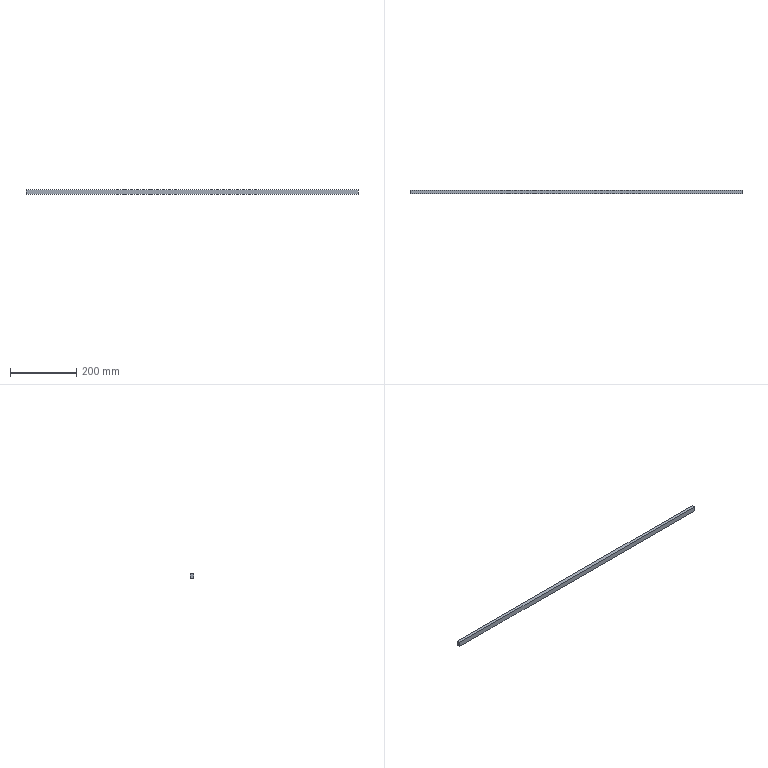Part | SolidWorks | features BaseBody 1, MoveFace 1 | 1 solid | 6 faces | box 1000 x 10 x 15 mm | volume 150000 mm3 | plane 6
STEP:
#1=CARTESIAN_POINT('',(225.,-60.,1490.));
#2=VERTEX_POINT('',#1);
#3=CARTESIAN_POINT('',(225.,-50.,1490.));
#4=VERTEX_POINT('',#3);
#5=CARTESIAN_POINT('',(225.,-55.,1490.));
#6=DIRECTION('',(0.,1.,0.));
#7=VECTOR('',#6,1000.);
#8=LINE('',#5,#7);
#9=EDGE_CURVE('',#2,#4,#8,.T.);
#10=ORIENTED_EDGE('',*,*,#9,.F.);
#11=CARTESIAN_POINT('',(225.,-60.,1475.));
#12=VERTEX_POINT('',#11);
#13=CARTESIAN_POINT('',(225.,-60.,1482.5));
#14=DIRECTION('',(0.,0.,1.));
#15=VECTOR('',#14,1000.);
#16=LINE('',#13,#15);
#17=EDGE_CURVE('',#12,#2,#16,.T.);
#18=ORIENTED_EDGE('',*,*,#17,.F.);
#19=CARTESIAN_POINT('',(225.,-50.,1475.));
#20=VERTEX_POINT('',#19);
#21=CARTESIAN_POINT('',(225.,-55.,1475.));
#22=DIRECTION('',(0.,-1.,0.));
#23=VECTOR('',#22,1000.);
#24=LINE('',#21,#23);
#25=EDGE_CURVE('',#20,#12,#24,.T.);
#26=ORIENTED_EDGE('',*,*,#25,.F.);
#27=CARTESIAN_POINT('',(225.,-50.,1482.5));
#28=DIRECTION('',(0.,0.,-1.));
#29=VECTOR('',#28,1000.);
#30=LINE('',#27,#29);
#31=EDGE_CURVE('',#4,#20,#30,.T.);
#32=ORIENTED_EDGE('',*,*,#31,.F.);
#33=EDGE_LOOP('',(#10,#18,#26,#32));
#34=FACE_OUTER_BOUND('',#33,.T.);
#35=CARTESIAN_POINT('',(225.,-65.003,1469.997));
#36=DIRECTION('',(-1.,0.,0.));
#37=DIRECTION('',(0.,0.,1.));
#38=AXIS2_PLACEMENT_3D('',#35,#36,#37);
#39=PLANE('',#38);
#40=ADVANCED_FACE('',(#34),#39,.F.);
#41=CARTESIAN_POINT('',(-775.,-50.,1475.));
#42=VERTEX_POINT('',#41);
#43=CARTESIAN_POINT('',(-775.,-50.,1490.));
#44=VERTEX_POINT('',#43);
#45=CARTESIAN_POINT('',(-775.,-50.,1482.5));
#46=DIRECTION('',(0.,0.,1.));
#47=VECTOR('',#46,1000.);
#48=LINE('',#45,#47);
#49=EDGE_CURVE('',#42,#44,#48,.T.);
#50=ORIENTED_EDGE('',*,*,#49,.T.);
#51=CARTESIAN_POINT('',(-525.,-50.,1490.));
#52=DIRECTION('',(1.,0.,0.));
#53=VECTOR('',#52,1000.);
#54=LINE('',#51,#53);
#55=EDGE_CURVE('',#44,#4,#54,.T.);
#56=ORIENTED_EDGE('',*,*,#55,.T.);
#57=ORIENTED_EDGE('',*,*,#31,.T.);
#58=CARTESIAN_POINT('',(-525.,-50.,1475.));
#59=DIRECTION('',(-1.,0.,0.));
#60=VECTOR('',#59,1000.);
#61=LINE('',#58,#60);
#62=EDGE_CURVE('',#20,#42,#61,.T.);
#63=ORIENTED_EDGE('',*,*,#62,.T.);
#64=EDGE_LOOP('',(#50,#56,#57,#63));
#65=FACE_OUTER_BOUND('',#64,.T.);
#66=CARTESIAN_POINT('',(-265.,-50.,1495.003));
#67=DIRECTION('',(0.,1.,0.));
#68=DIRECTION('',(0.,0.,-1.));
#69=AXIS2_PLACEMENT_3D('',#66,#67,#68);
#70=PLANE('',#69);
#71=ADVANCED_FACE('',(#65),#70,.T.);
#72=CARTESIAN_POINT('',(-775.,-60.,1490.));
#73=VERTEX_POINT('',#72);
#74=CARTESIAN_POINT('',(-775.,-55.,1490.));
#75=DIRECTION('',(0.,-1.,0.));
#76=VECTOR('',#75,1000.);
#77=LINE('',#74,#76);
#78=EDGE_CURVE('',#44,#73,#77,.T.);
#79=ORIENTED_EDGE('',*,*,#78,.T.);
#80=CARTESIAN_POINT('',(-525.,-60.,1490.));
#81=DIRECTION('',(1.,0.,0.));
#82=VECTOR('',#81,1000.);
#83=LINE('',#80,#82);
#84=EDGE_CURVE('',#73,#2,#83,.T.);
#85=ORIENTED_EDGE('',*,*,#84,.T.);
#86=ORIENTED_EDGE('',*,*,#9,.T.);
#87=ORIENTED_EDGE('',*,*,#55,.F.);
#88=EDGE_LOOP('',(#79,#85,#86,#87));
#89=FACE_OUTER_BOUND('',#88,.T.);
#90=CARTESIAN_POINT('',(-265.,-65.003,1490.));
#91=DIRECTION('',(0.,0.,1.));
#92=DIRECTION('',(0.,1.,0.));
#93=AXIS2_PLACEMENT_3D('',#90,#91,#92);
#94=PLANE('',#93);
#95=ADVANCED_FACE('',(#89),#94,.T.);
#96=CARTESIAN_POINT('',(-775.,-60.,1475.));
#97=VERTEX_POINT('',#96);
#98=CARTESIAN_POINT('',(-775.,-60.,1482.5));
#99=DIRECTION('',(0.,0.,-1.));
#100=VECTOR('',#99,1000.);
#101=LINE('',#98,#100);
#102=EDGE_CURVE('',#73,#97,#101,.T.);
#103=ORIENTED_EDGE('',*,*,#102,.T.);
#104=CARTESIAN_POINT('',(-525.,-60.,1475.));
#105=DIRECTION('',(1.,0.,0.));
#106=VECTOR('',#105,1000.);
#107=LINE('',#104,#106);
#108=EDGE_CURVE('',#97,#12,#107,.T.);
#109=ORIENTED_EDGE('',*,*,#108,.T.);
#110=ORIENTED_EDGE('',*,*,#17,.T.);
#111=ORIENTED_EDGE('',*,*,#84,.F.);
#112=EDGE_LOOP('',(#103,#109,#110,#111));
#113=FACE_OUTER_BOUND('',#112,.T.);
#114=CARTESIAN_POINT('',(-265.,-60.,1469.997));
#115=DIRECTION('',(0.,-1.,0.));
#116=DIRECTION('',(0.,0.,1.));
#117=AXIS2_PLACEMENT_3D('',#114,#115,#116);
#118=PLANE('',#117);
#119=ADVANCED_FACE('',(#113),#118,.T.);
#120=CARTESIAN_POINT('',(-775.,-55.,1475.));
#121=DIRECTION('',(0.,1.,0.));
#122=VECTOR('',#121,1000.);
#123=LINE('',#120,#122);
#124=EDGE_CURVE('',#97,#42,#123,.T.);
#125=ORIENTED_EDGE('',*,*,#124,.T.);
#126=ORIENTED_EDGE('',*,*,#62,.F.);
#127=ORIENTED_EDGE('',*,*,#25,.T.);
#128=ORIENTED_EDGE('',*,*,#108,.F.);
#129=EDGE_LOOP('',(#125,#126,#127,#128));
#130=FACE_OUTER_BOUND('',#129,.T.);
#131=CARTESIAN_POINT('',(-265.,-44.997,1475.));
#132=DIRECTION('',(0.,0.,-1.));
#133=DIRECTION('',(0.,-1.,0.));
#134=AXIS2_PLACEMENT_3D('',#131,#132,#133);
#135=PLANE('',#134);
#136=ADVANCED_FACE('',(#130),#135,.T.);
#137=ORIENTED_EDGE('',*,*,#78,.F.);
#138=ORIENTED_EDGE('',*,*,#49,.F.);
#139=ORIENTED_EDGE('',*,*,#124,.F.);
#140=ORIENTED_EDGE('',*,*,#102,.F.);
#141=EDGE_LOOP('',(#137,#138,#139,#140));
#142=FACE_OUTER_BOUND('',#141,.T.);
#143=CARTESIAN_POINT('',(-775.,-65.003,1469.997));
#144=DIRECTION('',(-1.,0.,0.));
#145=DIRECTION('',(0.,0.,1.));
#146=AXIS2_PLACEMENT_3D('',#143,#144,#145);
#147=PLANE('',#146);
#148=ADVANCED_FACE('',(#142),#147,.T.);
#149=CLOSED_SHELL('',(#40,#71,#95,#119,#136,#148));
#150=MANIFOLD_SOLID_BREP('',#149);
#151=CARTESIAN_POINT('',(0.,0.,0.));
#152=DIRECTION('',(0.,0.,1.));
#153=DIRECTION('',(1.,0.,0.));
#154=AXIS2_PLACEMENT_3D('',#151,#152,#153);
#155=(LENGTH_UNIT()NAMED_UNIT(*)SI_UNIT(.MILLI.,.METRE.));
#156=UNCERTAINTY_MEASURE_WITH_UNIT(LENGTH_MEASURE(0.00001),#155,'','');
#157=(NAMED_UNIT(*)PLANE_ANGLE_UNIT()SI_UNIT($,.RADIAN.));
#158=(NAMED_UNIT(*)SI_UNIT($,.STERADIAN.)SOLID_ANGLE_UNIT());
#159=(GEOMETRIC_REPRESENTATION_CONTEXT(3)GLOBAL_UNCERTAINTY_ASSIGNED_CONTEXT((#156))GLOBAL_UNIT_ASSIGNED_CONTEXT((#155,#157,#158))REPRESENTATION_CONTEXT('',''));
#160=ADVANCED_BREP_SHAPE_REPRESENTATION('',(#150,#154),#159);